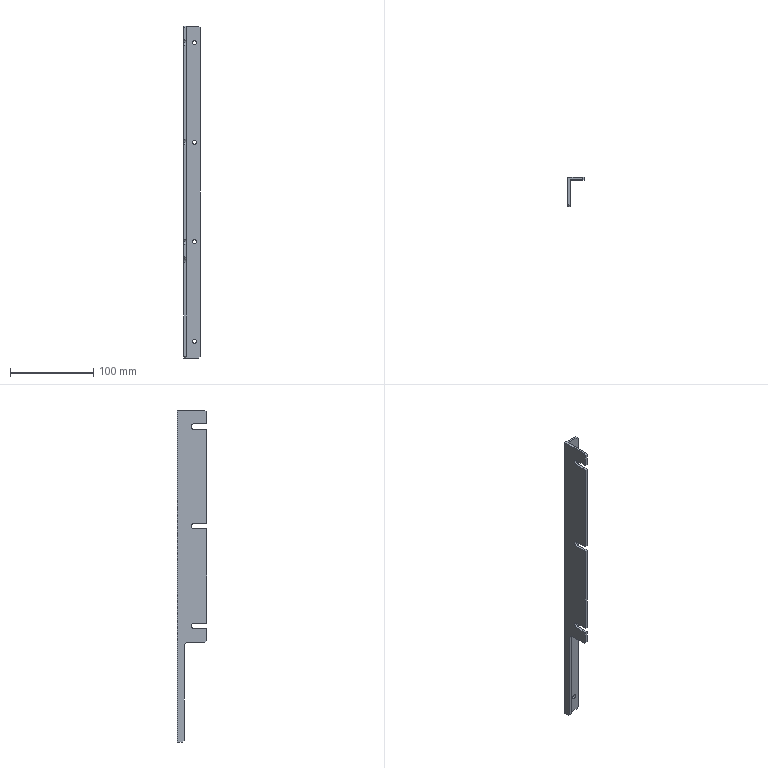Part | SolidWorks | features BaseBody 1 | 1 solid | 39 faces | box 20 x 35 x 400 mm | volume 51386 mm3 | plane 24 | cylinder 15 | commonest cylinder face diameters 5 x8 6.6 x6 10 x1
STEP:
#1=CARTESIAN_POINT('',(13.,32.,377.5));
#2=VERTEX_POINT('',#1);
#3=CARTESIAN_POINT('',(13.,32.,382.5));
#4=VERTEX_POINT('',#3);
#5=CARTESIAN_POINT('',(13.,32.,380.));
#6=DIRECTION('',(0.,1.,0.));
#7=DIRECTION('',(0.,0.,1.));
#8=AXIS2_PLACEMENT_3D('',#5,#6,#7);
#9=CIRCLE('',#8,2.5);
#10=EDGE_CURVE('',#2,#4,#9,.T.);
#11=ORIENTED_EDGE('',*,*,#10,.F.);
#12=CARTESIAN_POINT('',(13.,35.,377.5));
#13=VERTEX_POINT('',#12);
#14=CARTESIAN_POINT('',(13.,35.,377.5));
#15=DIRECTION('',(0.,1.,0.));
#16=VECTOR('',#15,1000.);
#17=LINE('',#14,#16);
#18=EDGE_CURVE('',#2,#13,#17,.T.);
#19=ORIENTED_EDGE('',*,*,#18,.T.);
#20=CARTESIAN_POINT('',(13.,35.,382.5));
#21=VERTEX_POINT('',#20);
#22=CARTESIAN_POINT('',(13.,35.,380.));
#23=DIRECTION('',(0.,1.,0.));
#24=DIRECTION('',(0.,0.,1.));
#25=AXIS2_PLACEMENT_3D('',#22,#23,#24);
#26=CIRCLE('',#25,2.5);
#27=EDGE_CURVE('',#13,#21,#26,.T.);
#28=ORIENTED_EDGE('',*,*,#27,.T.);
#29=CARTESIAN_POINT('',(13.,35.,382.5));
#30=DIRECTION('',(0.,1.,0.));
#31=VECTOR('',#30,1000.);
#32=LINE('',#29,#31);
#33=EDGE_CURVE('',#4,#21,#32,.T.);
#34=ORIENTED_EDGE('',*,*,#33,.F.);
#35=EDGE_LOOP('',(#11,#19,#28,#34));
#36=FACE_OUTER_BOUND('',#35,.T.);
#37=CARTESIAN_POINT('',(13.,35.,380.));
#38=DIRECTION('',(0.,1.,0.));
#39=DIRECTION('',(0.,0.,1.));
#40=AXIS2_PLACEMENT_3D('',#37,#38,#39);
#41=CYLINDRICAL_SURFACE('',#40,2.5);
#42=ADVANCED_FACE('',(#36),#41,.F.);
#43=CARTESIAN_POINT('',(13.,32.,257.5));
#44=VERTEX_POINT('',#43);
#45=CARTESIAN_POINT('',(13.,32.,262.5));
#46=VERTEX_POINT('',#45);
#47=CARTESIAN_POINT('',(13.,32.,260.));
#48=DIRECTION('',(0.,1.,0.));
#49=DIRECTION('',(0.,0.,1.));
#50=AXIS2_PLACEMENT_3D('',#47,#48,#49);
#51=CIRCLE('',#50,2.5);
#52=EDGE_CURVE('',#44,#46,#51,.T.);
#53=ORIENTED_EDGE('',*,*,#52,.F.);
#54=CARTESIAN_POINT('',(13.,35.,257.5));
#55=VERTEX_POINT('',#54);
#56=CARTESIAN_POINT('',(13.,35.,257.5));
#57=DIRECTION('',(0.,1.,0.));
#58=VECTOR('',#57,1000.);
#59=LINE('',#56,#58);
#60=EDGE_CURVE('',#44,#55,#59,.T.);
#61=ORIENTED_EDGE('',*,*,#60,.T.);
#62=CARTESIAN_POINT('',(13.,35.,262.5));
#63=VERTEX_POINT('',#62);
#64=CARTESIAN_POINT('',(13.,35.,260.));
#65=DIRECTION('',(0.,1.,0.));
#66=DIRECTION('',(0.,0.,1.));
#67=AXIS2_PLACEMENT_3D('',#64,#65,#66);
#68=CIRCLE('',#67,2.5);
#69=EDGE_CURVE('',#55,#63,#68,.T.);
#70=ORIENTED_EDGE('',*,*,#69,.T.);
#71=CARTESIAN_POINT('',(13.,35.,262.5));
#72=DIRECTION('',(0.,1.,0.));
#73=VECTOR('',#72,1000.);
#74=LINE('',#71,#73);
#75=EDGE_CURVE('',#46,#63,#74,.T.);
#76=ORIENTED_EDGE('',*,*,#75,.F.);
#77=EDGE_LOOP('',(#53,#61,#70,#76));
#78=FACE_OUTER_BOUND('',#77,.T.);
#79=CARTESIAN_POINT('',(13.,35.,260.));
#80=DIRECTION('',(0.,1.,0.));
#81=DIRECTION('',(0.,0.,1.));
#82=AXIS2_PLACEMENT_3D('',#79,#80,#81);
#83=CYLINDRICAL_SURFACE('',#82,2.5);
#84=ADVANCED_FACE('',(#78),#83,.F.);
#85=CARTESIAN_POINT('',(13.,32.,137.5));
#86=VERTEX_POINT('',#85);
#87=CARTESIAN_POINT('',(13.,32.,142.5));
#88=VERTEX_POINT('',#87);
#89=CARTESIAN_POINT('',(13.,32.,140.));
#90=DIRECTION('',(0.,1.,0.));
#91=DIRECTION('',(0.,0.,1.));
#92=AXIS2_PLACEMENT_3D('',#89,#90,#91);
#93=CIRCLE('',#92,2.5);
#94=EDGE_CURVE('',#86,#88,#93,.T.);
#95=ORIENTED_EDGE('',*,*,#94,.F.);
#96=CARTESIAN_POINT('',(13.,35.,137.5));
#97=VERTEX_POINT('',#96);
#98=CARTESIAN_POINT('',(13.,35.,137.5));
#99=DIRECTION('',(0.,1.,0.));
#100=VECTOR('',#99,1000.);
#101=LINE('',#98,#100);
#102=EDGE_CURVE('',#86,#97,#101,.T.);
#103=ORIENTED_EDGE('',*,*,#102,.T.);
#104=CARTESIAN_POINT('',(13.,35.,142.5));
#105=VERTEX_POINT('',#104);
#106=CARTESIAN_POINT('',(13.,35.,140.));
#107=DIRECTION('',(0.,1.,0.));
#108=DIRECTION('',(0.,0.,1.));
#109=AXIS2_PLACEMENT_3D('',#106,#107,#108);
#110=CIRCLE('',#109,2.5);
#111=EDGE_CURVE('',#97,#105,#110,.T.);
#112=ORIENTED_EDGE('',*,*,#111,.T.);
#113=CARTESIAN_POINT('',(13.,35.,142.5));
#114=DIRECTION('',(0.,1.,0.));
#115=VECTOR('',#114,1000.);
#116=LINE('',#113,#115);
#117=EDGE_CURVE('',#88,#105,#116,.T.);
#118=ORIENTED_EDGE('',*,*,#117,.F.);
#119=EDGE_LOOP('',(#95,#103,#112,#118));
#120=FACE_OUTER_BOUND('',#119,.T.);
#121=CARTESIAN_POINT('',(13.,35.,140.));
#122=DIRECTION('',(0.,1.,0.));
#123=DIRECTION('',(0.,0.,1.));
#124=AXIS2_PLACEMENT_3D('',#121,#122,#123);
#125=CYLINDRICAL_SURFACE('',#124,2.5);
#126=ADVANCED_FACE('',(#120),#125,.F.);
#127=CARTESIAN_POINT('',(13.,32.,17.5));
#128=VERTEX_POINT('',#127);
#129=CARTESIAN_POINT('',(13.,32.,22.5));
#130=VERTEX_POINT('',#129);
#131=CARTESIAN_POINT('',(13.,32.,20.));
#132=DIRECTION('',(0.,1.,0.));
#133=DIRECTION('',(0.,0.,1.));
#134=AXIS2_PLACEMENT_3D('',#131,#132,#133);
#135=CIRCLE('',#134,2.5);
#136=EDGE_CURVE('',#128,#130,#135,.T.);
#137=ORIENTED_EDGE('',*,*,#136,.F.);
#138=CARTESIAN_POINT('',(13.,35.,17.5));
#139=VERTEX_POINT('',#138);
#140=CARTESIAN_POINT('',(13.,35.,17.5));
#141=DIRECTION('',(0.,1.,0.));
#142=VECTOR('',#141,1000.);
#143=LINE('',#140,#142);
#144=EDGE_CURVE('',#128,#139,#143,.T.);
#145=ORIENTED_EDGE('',*,*,#144,.T.);
#146=CARTESIAN_POINT('',(13.,35.,22.5));
#147=VERTEX_POINT('',#146);
#148=CARTESIAN_POINT('',(13.,35.,20.));
#149=DIRECTION('',(0.,1.,0.));
#150=DIRECTION('',(0.,0.,1.));
#151=AXIS2_PLACEMENT_3D('',#148,#149,#150);
#152=CIRCLE('',#151,2.5);
#153=EDGE_CURVE('',#139,#147,#152,.T.);
#154=ORIENTED_EDGE('',*,*,#153,.T.);
#155=CARTESIAN_POINT('',(13.,35.,22.5));
#156=DIRECTION('',(0.,1.,0.));
#157=VECTOR('',#156,1000.);
#158=LINE('',#155,#157);
#159=EDGE_CURVE('',#130,#147,#158,.T.);
#160=ORIENTED_EDGE('',*,*,#159,.F.);
#161=EDGE_LOOP('',(#137,#145,#154,#160));
#162=FACE_OUTER_BOUND('',#161,.T.);
#163=CARTESIAN_POINT('',(13.,35.,20.));
#164=DIRECTION('',(0.,1.,0.));
#165=DIRECTION('',(0.,0.,1.));
#166=AXIS2_PLACEMENT_3D('',#163,#164,#165);
#167=CYLINDRICAL_SURFACE('',#166,2.5);
#168=ADVANCED_FACE('',(#162),#167,.F.);
#169=CARTESIAN_POINT('',(0.,18.3,140.));
#170=VERTEX_POINT('',#169);
#171=CARTESIAN_POINT('',(0.,15.,143.3));
#172=VERTEX_POINT('',#171);
#173=CARTESIAN_POINT('',(0.,15.,140.));
#174=DIRECTION('',(1.,0.,0.));
#175=DIRECTION('',(0.,1.,0.));
#176=AXIS2_PLACEMENT_3D('',#173,#174,#175);
#177=CIRCLE('',#176,3.3);
#178=EDGE_CURVE('',#170,#172,#177,.T.);
#179=ORIENTED_EDGE('',*,*,#178,.F.);
#180=CARTESIAN_POINT('',(3.,18.3,140.));
#181=VERTEX_POINT('',#180);
#182=CARTESIAN_POINT('',(0.,18.3,140.));
#183=DIRECTION('',(1.,0.,0.));
#184=VECTOR('',#183,1000.);
#185=LINE('',#182,#184);
#186=EDGE_CURVE('',#170,#181,#185,.T.);
#187=ORIENTED_EDGE('',*,*,#186,.T.);
#188=CARTESIAN_POINT('',(3.,15.,143.3));
#189=VERTEX_POINT('',#188);
#190=CARTESIAN_POINT('',(3.,15.,140.));
#191=DIRECTION('',(1.,0.,0.));
#192=DIRECTION('',(0.,1.,0.));
#193=AXIS2_PLACEMENT_3D('',#190,#191,#192);
#194=CIRCLE('',#193,3.3);
#195=EDGE_CURVE('',#181,#189,#194,.T.);
#196=ORIENTED_EDGE('',*,*,#195,.T.);
#197=CARTESIAN_POINT('',(0.,15.,143.3));
#198=DIRECTION('',(1.,0.,0.));
#199=VECTOR('',#198,1000.);
#200=LINE('',#197,#199);
#201=EDGE_CURVE('',#172,#189,#200,.T.);
#202=ORIENTED_EDGE('',*,*,#201,.F.);
#203=EDGE_LOOP('',(#179,#187,#196,#202));
#204=FACE_OUTER_BOUND('',#203,.T.);
#205=CARTESIAN_POINT('',(0.,15.,140.));
#206=DIRECTION('',(1.,0.,0.));
#207=DIRECTION('',(0.,1.,0.));
#208=AXIS2_PLACEMENT_3D('',#205,#206,#207);
#209=CYLINDRICAL_SURFACE('',#208,3.3);
#210=ADVANCED_FACE('',(#204),#209,.F.);
#211=CARTESIAN_POINT('',(0.,18.3,380.));
#212=VERTEX_POINT('',#211);
#213=CARTESIAN_POINT('',(0.,15.,383.3));
#214=VERTEX_POINT('',#213);
#215=CARTESIAN_POINT('',(0.,15.,380.));
#216=DIRECTION('',(1.,0.,0.));
#217=DIRECTION('',(0.,1.,0.));
#218=AXIS2_PLACEMENT_3D('',#215,#216,#217);
#219=CIRCLE('',#218,3.3);
#220=EDGE_CURVE('',#212,#214,#219,.T.);
#221=ORIENTED_EDGE('',*,*,#220,.F.);
#222=CARTESIAN_POINT('',(3.,18.3,380.));
#223=VERTEX_POINT('',#222);
#224=CARTESIAN_POINT('',(0.,18.3,380.));
#225=DIRECTION('',(1.,0.,0.));
#226=VECTOR('',#225,1000.);
#227=LINE('',#224,#226);
#228=EDGE_CURVE('',#212,#223,#227,.T.);
#229=ORIENTED_EDGE('',*,*,#228,.T.);
#230=CARTESIAN_POINT('',(3.,15.,383.3));
#231=VERTEX_POINT('',#230);
#232=CARTESIAN_POINT('',(3.,15.,380.));
#233=DIRECTION('',(1.,0.,0.));
#234=DIRECTION('',(0.,1.,0.));
#235=AXIS2_PLACEMENT_3D('',#232,#233,#234);
#236=CIRCLE('',#235,3.3);
#237=EDGE_CURVE('',#223,#231,#236,.T.);
#238=ORIENTED_EDGE('',*,*,#237,.T.);
#239=CARTESIAN_POINT('',(0.,15.,383.3));
#240=DIRECTION('',(1.,0.,0.));
#241=VECTOR('',#240,1000.);
#242=LINE('',#239,#241);
#243=EDGE_CURVE('',#214,#231,#242,.T.);
#244=ORIENTED_EDGE('',*,*,#243,.F.);
#245=EDGE_LOOP('',(#221,#229,#238,#244));
#246=FACE_OUTER_BOUND('',#245,.T.);
#247=CARTESIAN_POINT('',(0.,15.,380.));
#248=DIRECTION('',(1.,0.,0.));
#249=DIRECTION('',(0.,1.,0.));
#250=AXIS2_PLACEMENT_3D('',#247,#248,#249);
#251=CYLINDRICAL_SURFACE('',#250,3.3);
#252=ADVANCED_FACE('',(#246),#251,.F.);
#253=CARTESIAN_POINT('',(0.,18.3,260.));
#254=VERTEX_POINT('',#253);
#255=CARTESIAN_POINT('',(0.,15.,263.3));
#256=VERTEX_POINT('',#255);
#257=CARTESIAN_POINT('',(0.,15.,260.));
#258=DIRECTION('',(1.,0.,0.));
#259=DIRECTION('',(0.,1.,0.));
#260=AXIS2_PLACEMENT_3D('',#257,#258,#259);
#261=CIRCLE('',#260,3.3);
#262=EDGE_CURVE('',#254,#256,#261,.T.);
#263=ORIENTED_EDGE('',*,*,#262,.F.);
#264=CARTESIAN_POINT('',(3.,18.3,260.));
#265=VERTEX_POINT('',#264);
#266=CARTESIAN_POINT('',(0.,18.3,260.));
#267=DIRECTION('',(1.,0.,0.));
#268=VECTOR('',#267,1000.);
#269=LINE('',#266,#268);
#270=EDGE_CURVE('',#254,#265,#269,.T.);
#271=ORIENTED_EDGE('',*,*,#270,.T.);
#272=CARTESIAN_POINT('',(3.,15.,263.3));
#273=VERTEX_POINT('',#272);
#274=CARTESIAN_POINT('',(3.,15.,260.));
#275=DIRECTION('',(1.,0.,0.));
#276=DIRECTION('',(0.,1.,0.));
#277=AXIS2_PLACEMENT_3D('',#274,#275,#276);
#278=CIRCLE('',#277,3.3);
#279=EDGE_CURVE('',#265,#273,#278,.T.);
#280=ORIENTED_EDGE('',*,*,#279,.T.);
#281=CARTESIAN_POINT('',(0.,15.,263.3));
#282=DIRECTION('',(1.,0.,0.));
#283=VECTOR('',#282,1000.);
#284=LINE('',#281,#283);
#285=EDGE_CURVE('',#256,#273,#284,.T.);
#286=ORIENTED_EDGE('',*,*,#285,.F.);
#287=EDGE_LOOP('',(#263,#271,#280,#286));
#288=FACE_OUTER_BOUND('',#287,.T.);
#289=CARTESIAN_POINT('',(0.,15.,260.));
#290=DIRECTION('',(1.,0.,0.));
#291=DIRECTION('',(0.,1.,0.));
#292=AXIS2_PLACEMENT_3D('',#289,#290,#291);
#293=CYLINDRICAL_SURFACE('',#292,3.3);
#294=ADVANCED_FACE('',(#288),#293,.F.);
#295=CARTESIAN_POINT('',(0.,27.,115.));
#296=VERTEX_POINT('',#295);
#297=CARTESIAN_POINT('',(0.,22.,120.));
#298=VERTEX_POINT('',#297);
#299=CARTESIAN_POINT('',(0.,22.,115.));
#300=DIRECTION('',(1.,0.,0.));
#301=DIRECTION('',(0.,0.,-1.));
#302=AXIS2_PLACEMENT_3D('',#299,#300,#301);
#303=CIRCLE('',#302,5.);
#304=EDGE_CURVE('',#296,#298,#303,.T.);
#305=ORIENTED_EDGE('',*,*,#304,.F.);
#306=CARTESIAN_POINT('',(3.,27.,115.));
#307=VERTEX_POINT('',#306);
#308=CARTESIAN_POINT('',(0.,27.,115.));
#309=DIRECTION('',(-1.,0.,0.));
#310=VECTOR('',#309,1000.);
#311=LINE('',#308,#310);
#312=EDGE_CURVE('',#307,#296,#311,.T.);
#313=ORIENTED_EDGE('',*,*,#312,.F.);
#314=CARTESIAN_POINT('',(3.,22.,120.));
#315=VERTEX_POINT('',#314);
#316=CARTESIAN_POINT('',(3.,22.,115.));
#317=DIRECTION('',(-1.,0.,0.));
#318=DIRECTION('',(0.,-1.,0.));
#319=AXIS2_PLACEMENT_3D('',#316,#317,#318);
#320=CIRCLE('',#319,5.);
#321=EDGE_CURVE('',#315,#307,#320,.T.);
#322=ORIENTED_EDGE('',*,*,#321,.F.);
#323=CARTESIAN_POINT('',(3.,22.,120.));
#324=DIRECTION('',(1.,0.,0.));
#325=VECTOR('',#324,1000.);
#326=LINE('',#323,#325);
#327=EDGE_CURVE('',#298,#315,#326,.T.);
#328=ORIENTED_EDGE('',*,*,#327,.F.);
#329=EDGE_LOOP('',(#305,#313,#322,#328));
#330=FACE_OUTER_BOUND('',#329,.T.);
#331=CARTESIAN_POINT('',(0.,22.,115.));
#332=DIRECTION('',(-1.,0.,0.));
#333=DIRECTION('',(0.,-1.,0.));
#334=AXIS2_PLACEMENT_3D('',#331,#332,#333);
#335=CYLINDRICAL_SURFACE('',#334,5.);
#336=ADVANCED_FACE('',(#330),#335,.F.);
#337=CARTESIAN_POINT('',(18.,32.,0.));
#338=VERTEX_POINT('',#337);
#339=CARTESIAN_POINT('',(20.,32.,2.));
#340=VERTEX_POINT('',#339);
#341=CARTESIAN_POINT('',(20.,32.,2.));
#342=DIRECTION('',(0.7071,0.,0.7071));
#343=VECTOR('',#342,1000.);
#344=LINE('',#341,#343);
#345=EDGE_CURVE('',#338,#340,#344,.T.);
#346=ORIENTED_EDGE('',*,*,#345,.F.);
#347=CARTESIAN_POINT('',(18.,35.,0.));
#348=VERTEX_POINT('',#347);
#349=CARTESIAN_POINT('',(18.,32.,0.));
#350=DIRECTION('',(0.,-1.,0.));
#351=VECTOR('',#350,1000.);
#352=LINE('',#349,#351);
#353=EDGE_CURVE('',#348,#338,#352,.T.);
#354=ORIENTED_EDGE('',*,*,#353,.F.);
#355=CARTESIAN_POINT('',(20.,35.,2.));
#356=VERTEX_POINT('',#355);
#357=CARTESIAN_POINT('',(20.,35.,2.));
#358=DIRECTION('',(-0.7071,0.,-0.7071));
#359=VECTOR('',#358,1000.);
#360=LINE('',#357,#359);
#361=EDGE_CURVE('',#356,#348,#360,.T.);
#362=ORIENTED_EDGE('',*,*,#361,.F.);
#363=CARTESIAN_POINT('',(20.,35.,2.));
#364=DIRECTION('',(0.,1.,0.));
#365=VECTOR('',#364,1000.);
#366=LINE('',#363,#365);
#367=EDGE_CURVE('',#340,#356,#366,.T.);
#368=ORIENTED_EDGE('',*,*,#367,.F.);
#369=EDGE_LOOP('',(#346,#354,#362,#368));
#370=FACE_OUTER_BOUND('',#369,.T.);
#371=CARTESIAN_POINT('',(20.,35.,2.));
#372=DIRECTION('',(0.7071,0.,-0.7071));
#373=DIRECTION('',(0.,-1.,0.));
#374=AXIS2_PLACEMENT_3D('',#371,#372,#373);
#375=PLANE('',#374);
#376=ADVANCED_FACE('',(#370),#375,.T.);
#377=CARTESIAN_POINT('',(0.,29.,0.));
#378=VERTEX_POINT('',#377);
#379=CARTESIAN_POINT('',(0.,27.,2.));
#380=VERTEX_POINT('',#379);
#381=CARTESIAN_POINT('',(0.,27.,2.));
#382=DIRECTION('',(0.,-0.7071,0.7071));
#383=VECTOR('',#382,1000.);
#384=LINE('',#381,#383);
#385=EDGE_CURVE('',#378,#380,#384,.T.);
#386=ORIENTED_EDGE('',*,*,#385,.F.);
#387=CARTESIAN_POINT('',(3.,29.,0.));
#388=VERTEX_POINT('',#387);
#389=CARTESIAN_POINT('',(0.,29.,0.));
#390=DIRECTION('',(-1.,0.,0.));
#391=VECTOR('',#390,1000.);
#392=LINE('',#389,#391);
#393=EDGE_CURVE('',#388,#378,#392,.T.);
#394=ORIENTED_EDGE('',*,*,#393,.F.);
#395=CARTESIAN_POINT('',(3.,27.,2.));
#396=VERTEX_POINT('',#395);
#397=CARTESIAN_POINT('',(3.,27.,2.));
#398=DIRECTION('',(0.,0.7071,-0.7071));
#399=VECTOR('',#398,1000.);
#400=LINE('',#397,#399);
#401=EDGE_CURVE('',#396,#388,#400,.T.);
#402=ORIENTED_EDGE('',*,*,#401,.F.);
#403=CARTESIAN_POINT('',(3.,27.,2.));
#404=DIRECTION('',(1.,0.,0.));
#405=VECTOR('',#404,1000.);
#406=LINE('',#403,#405);
#407=EDGE_CURVE('',#380,#396,#406,.T.);
#408=ORIENTED_EDGE('',*,*,#407,.F.);
#409=EDGE_LOOP('',(#386,#394,#402,#408));
#410=FACE_OUTER_BOUND('',#409,.T.);
#411=CARTESIAN_POINT('',(0.,27.,2.));
#412=DIRECTION('',(0.,-0.7071,-0.7071));
#413=DIRECTION('',(0.,-0.7071,0.7071));
#414=AXIS2_PLACEMENT_3D('',#411,#412,#413);
#415=PLANE('',#414);
#416=ADVANCED_FACE('',(#410),#415,.T.);
#417=CARTESIAN_POINT('',(0.,2.,120.));
#418=VERTEX_POINT('',#417);
#419=CARTESIAN_POINT('',(0.,0.,122.));
#420=VERTEX_POINT('',#419);
#421=CARTESIAN_POINT('',(0.,0.,122.));
#422=DIRECTION('',(0.,-0.7071,0.7071));
#423=VECTOR('',#422,1000.);
#424=LINE('',#421,#423);
#425=EDGE_CURVE('',#418,#420,#424,.T.);
#426=ORIENTED_EDGE('',*,*,#425,.F.);
#427=CARTESIAN_POINT('',(3.,2.,120.));
#428=VERTEX_POINT('',#427);
#429=CARTESIAN_POINT('',(0.,2.,120.));
#430=DIRECTION('',(-1.,0.,0.));
#431=VECTOR('',#430,1000.);
#432=LINE('',#429,#431);
#433=EDGE_CURVE('',#428,#418,#432,.T.);
#434=ORIENTED_EDGE('',*,*,#433,.F.);
#435=CARTESIAN_POINT('',(3.,0.,122.));
#436=VERTEX_POINT('',#435);
#437=CARTESIAN_POINT('',(3.,0.,122.));
#438=DIRECTION('',(0.,0.7071,-0.7071));
#439=VECTOR('',#438,1000.);
#440=LINE('',#437,#439);
#441=EDGE_CURVE('',#436,#428,#440,.T.);
#442=ORIENTED_EDGE('',*,*,#441,.F.);
#443=CARTESIAN_POINT('',(3.,0.,122.));
#444=DIRECTION('',(1.,0.,0.));
#445=VECTOR('',#444,1000.);
#446=LINE('',#443,#445);
#447=EDGE_CURVE('',#420,#436,#446,.T.);
#448=ORIENTED_EDGE('',*,*,#447,.F.);
#449=EDGE_LOOP('',(#426,#434,#442,#448));
#450=FACE_OUTER_BOUND('',#449,.T.);
#451=CARTESIAN_POINT('',(3.,0.,122.));
#452=DIRECTION('',(0.,0.7071,0.7071));
#453=DIRECTION('',(1.,0.,0.));
#454=AXIS2_PLACEMENT_3D('',#451,#452,#453);
#455=PLANE('',#454);
#456=ADVANCED_FACE('',(#450),#455,.F.);
#457=CARTESIAN_POINT('',(0.,0.,398.));
#458=VERTEX_POINT('',#457);
#459=CARTESIAN_POINT('',(0.,2.,400.));
#460=VERTEX_POINT('',#459);
#461=CARTESIAN_POINT('',(0.,2.,400.));
#462=DIRECTION('',(0.,0.7071,0.7071));
#463=VECTOR('',#462,1000.);
#464=LINE('',#461,#463);
#465=EDGE_CURVE('',#458,#460,#464,.T.);
#466=ORIENTED_EDGE('',*,*,#465,.F.);
#467=CARTESIAN_POINT('',(3.,0.,398.));
#468=VERTEX_POINT('',#467);
#469=CARTESIAN_POINT('',(3.,0.,398.));
#470=DIRECTION('',(-1.,0.,0.));
#471=VECTOR('',#470,1000.);
#472=LINE('',#469,#471);
#473=EDGE_CURVE('',#468,#458,#472,.T.);
#474=ORIENTED_EDGE('',*,*,#473,.F.);
#475=CARTESIAN_POINT('',(3.,2.,400.));
#476=VERTEX_POINT('',#475);
#477=CARTESIAN_POINT('',(3.,2.,400.));
#478=DIRECTION('',(0.,-0.7071,-0.7071));
#479=VECTOR('',#478,1000.);
#480=LINE('',#477,#479);
#481=EDGE_CURVE('',#476,#468,#480,.T.);
#482=ORIENTED_EDGE('',*,*,#481,.F.);
#483=CARTESIAN_POINT('',(0.,2.,400.));
#484=DIRECTION('',(1.,0.,0.));
#485=VECTOR('',#484,1000.);
#486=LINE('',#483,#485);
#487=EDGE_CURVE('',#460,#476,#486,.T.);
#488=ORIENTED_EDGE('',*,*,#487,.F.);
#489=EDGE_LOOP('',(#466,#474,#482,#488));
#490=FACE_OUTER_BOUND('',#489,.T.);
#491=CARTESIAN_POINT('',(0.,2.,400.));
#492=DIRECTION('',(0.,0.7071,-0.7071));
#493=DIRECTION('',(-1.,0.,0.));
#494=AXIS2_PLACEMENT_3D('',#491,#492,#493);
#495=PLANE('',#494);
#496=ADVANCED_FACE('',(#490),#495,.F.);
#497=CARTESIAN_POINT('',(20.,32.,398.));
#498=VERTEX_POINT('',#497);
#499=CARTESIAN_POINT('',(18.,32.,400.));
#500=VERTEX_POINT('',#499);
#501=CARTESIAN_POINT('',(18.,32.,400.));
#502=DIRECTION('',(-0.7071,0.,0.7071));
#503=VECTOR('',#502,1000.);
#504=LINE('',#501,#503);
#505=EDGE_CURVE('',#498,#500,#504,.T.);
#506=ORIENTED_EDGE('',*,*,#505,.F.);
#507=CARTESIAN_POINT('',(20.,35.,398.));
#508=VERTEX_POINT('',#507);
#509=CARTESIAN_POINT('',(20.,35.,398.));
#510=DIRECTION('',(0.,-1.,0.));
#511=VECTOR('',#510,1000.);
#512=LINE('',#509,#511);
#513=EDGE_CURVE('',#508,#498,#512,.T.);
#514=ORIENTED_EDGE('',*,*,#513,.F.);
#515=CARTESIAN_POINT('',(18.,35.,400.));
#516=VERTEX_POINT('',#515);
#517=CARTESIAN_POINT('',(18.,35.,400.));
#518=DIRECTION('',(0.7071,0.,-0.7071));
#519=VECTOR('',#518,1000.);
#520=LINE('',#517,#519);
#521=EDGE_CURVE('',#516,#508,#520,.T.);
#522=ORIENTED_EDGE('',*,*,#521,.F.);
#523=CARTESIAN_POINT('',(18.,0.,400.));
#524=DIRECTION('',(0.,1.,0.));
#525=VECTOR('',#524,1000.);
#526=LINE('',#523,#525);
#527=EDGE_CURVE('',#500,#516,#526,.T.);
#528=ORIENTED_EDGE('',*,*,#527,.F.);
#529=EDGE_LOOP('',(#506,#514,#522,#528));
#530=FACE_OUTER_BOUND('',#529,.T.);
#531=CARTESIAN_POINT('',(18.,0.,400.));
#532=DIRECTION('',(-0.7071,0.,-0.7071));
#533=DIRECTION('',(-0.7071,0.,0.7071));
#534=AXIS2_PLACEMENT_3D('',#531,#532,#533);
#535=PLANE('',#534);
#536=ADVANCED_FACE('',(#530),#535,.F.);
#537=CARTESIAN_POINT('',(3.,27.,0.));
#538=DIRECTION('',(0.,0.,1.));
#539=VECTOR('',#538,1000.);
#540=LINE('',#537,#539);
#541=EDGE_CURVE('',#396,#307,#540,.T.);
#542=ORIENTED_EDGE('',*,*,#541,.T.);
#543=ORIENTED_EDGE('',*,*,#312,.T.);
#544=CARTESIAN_POINT('',(0.,27.,0.));
#545=DIRECTION('',(0.,0.,1.));
#546=VECTOR('',#545,1000.);
#547=LINE('',#544,#546);
#548=EDGE_CURVE('',#380,#296,#547,.T.);
#549=ORIENTED_EDGE('',*,*,#548,.F.);
#550=ORIENTED_EDGE('',*,*,#407,.T.);
#551=EDGE_LOOP('',(#542,#543,#549,#550));
#552=FACE_OUTER_BOUND('',#551,.T.);
#553=CARTESIAN_POINT('',(0.,27.,0.));
#554=DIRECTION('',(0.,1.,0.));
#555=DIRECTION('',(1.,0.,0.));
#556=AXIS2_PLACEMENT_3D('',#553,#554,#555);
#557=PLANE('',#556);
#558=ADVANCED_FACE('',(#552),#557,.F.);
#559=CARTESIAN_POINT('',(0.,0.,120.));
#560=DIRECTION('',(0.,-1.,0.));
#561=VECTOR('',#560,1000.);
#562=LINE('',#559,#561);
#563=EDGE_CURVE('',#298,#418,#562,.T.);
#564=ORIENTED_EDGE('',*,*,#563,.F.);
#565=ORIENTED_EDGE('',*,*,#327,.T.);
#566=CARTESIAN_POINT('',(3.,0.,120.));
#567=DIRECTION('',(0.,-1.,0.));
#568=VECTOR('',#567,1000.);
#569=LINE('',#566,#568);
#570=EDGE_CURVE('',#315,#428,#569,.T.);
#571=ORIENTED_EDGE('',*,*,#570,.T.);
#572=ORIENTED_EDGE('',*,*,#433,.T.);
#573=EDGE_LOOP('',(#564,#565,#571,#572));
#574=FACE_OUTER_BOUND('',#573,.T.);
#575=CARTESIAN_POINT('',(0.,0.,120.));
#576=DIRECTION('',(0.,0.,1.));
#577=DIRECTION('',(1.,0.,0.));
#578=AXIS2_PLACEMENT_3D('',#575,#576,#577);
#579=PLANE('',#578);
#580=ADVANCED_FACE('',(#574),#579,.F.);
#581=CARTESIAN_POINT('',(3.,0.,136.7));
#582=VERTEX_POINT('',#581);
#583=CARTESIAN_POINT('',(3.,15.,136.7));
#584=VERTEX_POINT('',#583);
#585=CARTESIAN_POINT('',(3.,0.,136.7));
#586=DIRECTION('',(0.,1.,0.));
#587=VECTOR('',#586,1000.);
#588=LINE('',#585,#587);
#589=EDGE_CURVE('',#582,#584,#588,.T.);
#590=ORIENTED_EDGE('',*,*,#589,.T.);
#591=CARTESIAN_POINT('',(0.,15.,136.7));
#592=VERTEX_POINT('',#591);
#593=CARTESIAN_POINT('',(0.,15.,136.7));
#594=DIRECTION('',(1.,0.,0.));
#595=VECTOR('',#594,1000.);
#596=LINE('',#593,#595);
#597=EDGE_CURVE('',#592,#584,#596,.T.);
#598=ORIENTED_EDGE('',*,*,#597,.F.);
#599=CARTESIAN_POINT('',(0.,0.,136.7));
#600=VERTEX_POINT('',#599);
#601=CARTESIAN_POINT('',(0.,0.,136.7));
#602=DIRECTION('',(0.,1.,0.));
#603=VECTOR('',#602,1000.);
#604=LINE('',#601,#603);
#605=EDGE_CURVE('',#600,#592,#604,.T.);
#606=ORIENTED_EDGE('',*,*,#605,.F.);
#607=CARTESIAN_POINT('',(0.,0.,136.7));
#608=DIRECTION('',(1.,0.,0.));
#609=VECTOR('',#608,1000.);
#610=LINE('',#607,#609);
#611=EDGE_CURVE('',#600,#582,#610,.T.);
#612=ORIENTED_EDGE('',*,*,#611,.T.);
#613=EDGE_LOOP('',(#590,#598,#606,#612));
#614=FACE_OUTER_BOUND('',#613,.T.);
#615=CARTESIAN_POINT('',(0.,0.,136.7));
#616=DIRECTION('',(0.,0.,-1.));
#617=DIRECTION('',(-1.,0.,0.));
#618=AXIS2_PLACEMENT_3D('',#615,#616,#617);
#619=PLANE('',#618);
#620=ADVANCED_FACE('',(#614),#619,.F.);
#621=CARTESIAN_POINT('',(3.,0.,143.3));
#622=VERTEX_POINT('',#621);
#623=CARTESIAN_POINT('',(3.,0.,143.3));
#624=DIRECTION('',(0.,-1.,0.));
#625=VECTOR('',#624,1000.);
#626=LINE('',#623,#625);
#627=EDGE_CURVE('',#189,#622,#626,.T.);
#628=ORIENTED_EDGE('',*,*,#627,.T.);
#629=CARTESIAN_POINT('',(0.,0.,143.3));
#630=VERTEX_POINT('',#629);
#631=CARTESIAN_POINT('',(0.,0.,143.3));
#632=DIRECTION('',(1.,0.,0.));
#633=VECTOR('',#632,1000.);
#634=LINE('',#631,#633);
#635=EDGE_CURVE('',#630,#622,#634,.T.);
#636=ORIENTED_EDGE('',*,*,#635,.F.);
#637=CARTESIAN_POINT('',(0.,0.,143.3));
#638=DIRECTION('',(0.,-1.,0.));
#639=VECTOR('',#638,1000.);
#640=LINE('',#637,#639);
#641=EDGE_CURVE('',#172,#630,#640,.T.);
#642=ORIENTED_EDGE('',*,*,#641,.F.);
#643=ORIENTED_EDGE('',*,*,#201,.T.);
#644=EDGE_LOOP('',(#628,#636,#642,#643));
#645=FACE_OUTER_BOUND('',#644,.T.);
#646=CARTESIAN_POINT('',(0.,0.,143.3));
#647=DIRECTION('',(0.,0.,1.));
#648=DIRECTION('',(0.,-1.,0.));
#649=AXIS2_PLACEMENT_3D('',#646,#647,#648);
#650=PLANE('',#649);
#651=ADVANCED_FACE('',(#645),#650,.F.);
#652=CARTESIAN_POINT('',(3.,0.,376.7));
#653=VERTEX_POINT('',#652);
#654=CARTESIAN_POINT('',(3.,15.,376.7));
#655=VERTEX_POINT('',#654);
#656=CARTESIAN_POINT('',(3.,0.,376.7));
#657=DIRECTION('',(0.,1.,0.));
#658=VECTOR('',#657,1000.);
#659=LINE('',#656,#658);
#660=EDGE_CURVE('',#653,#655,#659,.T.);
#661=ORIENTED_EDGE('',*,*,#660,.T.);
#662=CARTESIAN_POINT('',(0.,15.,376.7));
#663=VERTEX_POINT('',#662);
#664=CARTESIAN_POINT('',(0.,15.,376.7));
#665=DIRECTION('',(1.,0.,0.));
#666=VECTOR('',#665,1000.);
#667=LINE('',#664,#666);
#668=EDGE_CURVE('',#663,#655,#667,.T.);
#669=ORIENTED_EDGE('',*,*,#668,.F.);
#670=CARTESIAN_POINT('',(0.,0.,376.7));
#671=VERTEX_POINT('',#670);
#672=CARTESIAN_POINT('',(0.,0.,376.7));
#673=DIRECTION('',(0.,1.,0.));
#674=VECTOR('',#673,1000.);
#675=LINE('',#672,#674);
#676=EDGE_CURVE('',#671,#663,#675,.T.);
#677=ORIENTED_EDGE('',*,*,#676,.F.);
#678=CARTESIAN_POINT('',(0.,0.,376.7));
#679=DIRECTION('',(1.,0.,0.));
#680=VECTOR('',#679,1000.);
#681=LINE('',#678,#680);
#682=EDGE_CURVE('',#671,#653,#681,.T.);
#683=ORIENTED_EDGE('',*,*,#682,.T.);
#684=EDGE_LOOP('',(#661,#669,#677,#683));
#685=FACE_OUTER_BOUND('',#684,.T.);
#686=CARTESIAN_POINT('',(0.,0.,376.7));
#687=DIRECTION('',(0.,0.,-1.));
#688=DIRECTION('',(0.,-1.,0.));
#689=AXIS2_PLACEMENT_3D('',#686,#687,#688);
#690=PLANE('',#689);
#691=ADVANCED_FACE('',(#685),#690,.F.);
#692=CARTESIAN_POINT('',(3.,0.,383.3));
#693=VERTEX_POINT('',#692);
#694=CARTESIAN_POINT('',(3.,0.,383.3));
#695=DIRECTION('',(0.,-1.,0.));
#696=VECTOR('',#695,1000.);
#697=LINE('',#694,#696);
#698=EDGE_CURVE('',#231,#693,#697,.T.);
#699=ORIENTED_EDGE('',*,*,#698,.T.);
#700=CARTESIAN_POINT('',(0.,0.,383.3));
#701=VERTEX_POINT('',#700);
#702=CARTESIAN_POINT('',(0.,0.,383.3));
#703=DIRECTION('',(1.,0.,0.));
#704=VECTOR('',#703,1000.);
#705=LINE('',#702,#704);
#706=EDGE_CURVE('',#701,#693,#705,.T.);
#707=ORIENTED_EDGE('',*,*,#706,.F.);
#708=CARTESIAN_POINT('',(0.,0.,383.3));
#709=DIRECTION('',(0.,-1.,0.));
#710=VECTOR('',#709,1000.);
#711=LINE('',#708,#710);
#712=EDGE_CURVE('',#214,#701,#711,.T.);
#713=ORIENTED_EDGE('',*,*,#712,.F.);
#714=ORIENTED_EDGE('',*,*,#243,.T.);
#715=EDGE_LOOP('',(#699,#707,#713,#714));
#716=FACE_OUTER_BOUND('',#715,.T.);
#717=CARTESIAN_POINT('',(0.,0.,383.3));
#718=DIRECTION('',(0.,0.,1.));
#719=DIRECTION('',(0.,-1.,0.));
#720=AXIS2_PLACEMENT_3D('',#717,#718,#719);
#721=PLANE('',#720);
#722=ADVANCED_FACE('',(#716),#721,.F.);
#723=CARTESIAN_POINT('',(3.,0.,263.3));
#724=VERTEX_POINT('',#723);
#725=CARTESIAN_POINT('',(3.,15.,263.3));
#726=DIRECTION('',(0.,-1.,0.));
#727=VECTOR('',#726,1000.);
#728=LINE('',#725,#727);
#729=EDGE_CURVE('',#273,#724,#728,.T.);
#730=ORIENTED_EDGE('',*,*,#729,.T.);
#731=CARTESIAN_POINT('',(0.,0.,263.3));
#732=VERTEX_POINT('',#731);
#733=CARTESIAN_POINT('',(0.,0.,263.3));
#734=DIRECTION('',(1.,0.,0.));
#735=VECTOR('',#734,1000.);
#736=LINE('',#733,#735);
#737=EDGE_CURVE('',#732,#724,#736,.T.);
#738=ORIENTED_EDGE('',*,*,#737,.F.);
#739=CARTESIAN_POINT('',(0.,15.,263.3));
#740=DIRECTION('',(0.,-1.,0.));
#741=VECTOR('',#740,1000.);
#742=LINE('',#739,#741);
#743=EDGE_CURVE('',#256,#732,#742,.T.);
#744=ORIENTED_EDGE('',*,*,#743,.F.);
#745=ORIENTED_EDGE('',*,*,#285,.T.);
#746=EDGE_LOOP('',(#730,#738,#744,#745));
#747=FACE_OUTER_BOUND('',#746,.T.);
#748=CARTESIAN_POINT('',(0.,15.,263.3));
#749=DIRECTION('',(0.,0.,1.));
#750=DIRECTION('',(0.,-1.,0.));
#751=AXIS2_PLACEMENT_3D('',#748,#749,#750);
#752=PLANE('',#751);
#753=ADVANCED_FACE('',(#747),#752,.F.);
#754=CARTESIAN_POINT('',(3.,0.,256.7));
#755=VERTEX_POINT('',#754);
#756=CARTESIAN_POINT('',(3.,15.,256.7));
#757=VERTEX_POINT('',#756);
#758=CARTESIAN_POINT('',(3.,15.,256.7));
#759=DIRECTION('',(0.,1.,0.));
#760=VECTOR('',#759,1000.);
#761=LINE('',#758,#760);
#762=EDGE_CURVE('',#755,#757,#761,.T.);
#763=ORIENTED_EDGE('',*,*,#762,.T.);
#764=CARTESIAN_POINT('',(0.,15.,256.7));
#765=VERTEX_POINT('',#764);
#766=CARTESIAN_POINT('',(0.,15.,256.7));
#767=DIRECTION('',(1.,0.,0.));
#768=VECTOR('',#767,1000.);
#769=LINE('',#766,#768);
#770=EDGE_CURVE('',#765,#757,#769,.T.);
#771=ORIENTED_EDGE('',*,*,#770,.F.);
#772=CARTESIAN_POINT('',(0.,0.,256.7));
#773=VERTEX_POINT('',#772);
#774=CARTESIAN_POINT('',(0.,15.,256.7));
#775=DIRECTION('',(0.,1.,0.));
#776=VECTOR('',#775,1000.);
#777=LINE('',#774,#776);
#778=EDGE_CURVE('',#773,#765,#777,.T.);
#779=ORIENTED_EDGE('',*,*,#778,.F.);
#780=CARTESIAN_POINT('',(0.,0.,256.7));
#781=DIRECTION('',(1.,0.,0.));
#782=VECTOR('',#781,1000.);
#783=LINE('',#780,#782);
#784=EDGE_CURVE('',#773,#755,#783,.T.);
#785=ORIENTED_EDGE('',*,*,#784,.T.);
#786=EDGE_LOOP('',(#763,#771,#779,#785));
#787=FACE_OUTER_BOUND('',#786,.T.);
#788=CARTESIAN_POINT('',(0.,15.,256.7));
#789=DIRECTION('',(0.,0.,-1.));
#790=DIRECTION('',(-1.,0.,0.));
#791=AXIS2_PLACEMENT_3D('',#788,#789,#790);
#792=PLANE('',#791);
#793=ADVANCED_FACE('',(#787),#792,.F.);
#794=CARTESIAN_POINT('',(3.,32.,0.));
#795=VERTEX_POINT('',#794);
#796=CARTESIAN_POINT('',(3.,32.,0.));
#797=DIRECTION('',(0.,1.,0.));
#798=VECTOR('',#797,1000.);
#799=LINE('',#796,#798);
#800=EDGE_CURVE('',#388,#795,#799,.T.);
#801=ORIENTED_EDGE('',*,*,#800,.F.);
#802=ORIENTED_EDGE('',*,*,#393,.T.);
#803=CARTESIAN_POINT('',(0.,35.,0.));
#804=VERTEX_POINT('',#803);
#805=CARTESIAN_POINT('',(0.,0.,0.));
#806=DIRECTION('',(0.,-1.,0.));
#807=VECTOR('',#806,1000.);
#808=LINE('',#805,#807);
#809=EDGE_CURVE('',#804,#378,#808,.T.);
#810=ORIENTED_EDGE('',*,*,#809,.F.);
#811=CARTESIAN_POINT('',(0.,35.,0.));
#812=DIRECTION('',(-1.,0.,0.));
#813=VECTOR('',#812,1000.);
#814=LINE('',#811,#813);
#815=EDGE_CURVE('',#348,#804,#814,.T.);
#816=ORIENTED_EDGE('',*,*,#815,.F.);
#817=ORIENTED_EDGE('',*,*,#353,.T.);
#818=CARTESIAN_POINT('',(20.,32.,0.));
#819=DIRECTION('',(1.,0.,0.));
#820=VECTOR('',#819,1000.);
#821=LINE('',#818,#820);
#822=EDGE_CURVE('',#795,#338,#821,.T.);
#823=ORIENTED_EDGE('',*,*,#822,.F.);
#824=EDGE_LOOP('',(#801,#802,#810,#816,#817,#823));
#825=FACE_OUTER_BOUND('',#824,.T.);
#826=CARTESIAN_POINT('',(0.,0.,0.));
#827=DIRECTION('',(0.,0.,-1.));
#828=DIRECTION('',(0.,-1.,0.));
#829=AXIS2_PLACEMENT_3D('',#826,#827,#828);
#830=PLANE('',#829);
#831=ADVANCED_FACE('',(#825),#830,.T.);
#832=CARTESIAN_POINT('',(3.,32.,400.));
#833=VERTEX_POINT('',#832);
#834=CARTESIAN_POINT('',(20.,32.,400.));
#835=DIRECTION('',(1.,0.,0.));
#836=VECTOR('',#835,1000.);
#837=LINE('',#834,#836);
#838=EDGE_CURVE('',#833,#500,#837,.T.);
#839=ORIENTED_EDGE('',*,*,#838,.T.);
#840=ORIENTED_EDGE('',*,*,#527,.T.);
#841=CARTESIAN_POINT('',(0.,35.,400.));
#842=VERTEX_POINT('',#841);
#843=CARTESIAN_POINT('',(0.,35.,400.));
#844=DIRECTION('',(-1.,0.,0.));
#845=VECTOR('',#844,1000.);
#846=LINE('',#843,#845);
#847=EDGE_CURVE('',#516,#842,#846,.T.);
#848=ORIENTED_EDGE('',*,*,#847,.T.);
#849=CARTESIAN_POINT('',(0.,0.,400.));
#850=DIRECTION('',(0.,-1.,0.));
#851=VECTOR('',#850,1000.);
#852=LINE('',#849,#851);
#853=EDGE_CURVE('',#842,#460,#852,.T.);
#854=ORIENTED_EDGE('',*,*,#853,.T.);
#855=ORIENTED_EDGE('',*,*,#487,.T.);
#856=CARTESIAN_POINT('',(3.,32.,400.));
#857=DIRECTION('',(0.,1.,0.));
#858=VECTOR('',#857,1000.);
#859=LINE('',#856,#858);
#860=EDGE_CURVE('',#476,#833,#859,.T.);
#861=ORIENTED_EDGE('',*,*,#860,.T.);
#862=EDGE_LOOP('',(#839,#840,#848,#854,#855,#861));
#863=FACE_OUTER_BOUND('',#862,.T.);
#864=CARTESIAN_POINT('',(0.,0.,400.));
#865=DIRECTION('',(0.,0.,-1.));
#866=DIRECTION('',(0.,-1.,0.));
#867=AXIS2_PLACEMENT_3D('',#864,#865,#866);
#868=PLANE('',#867);
#869=ADVANCED_FACE('',(#863),#868,.F.);
#870=CARTESIAN_POINT('',(0.,0.,400.));
#871=DIRECTION('',(0.,0.,-1.));
#872=VECTOR('',#871,1000.);
#873=LINE('',#870,#872);
#874=EDGE_CURVE('',#458,#701,#873,.T.);
#875=ORIENTED_EDGE('',*,*,#874,.F.);
#876=ORIENTED_EDGE('',*,*,#465,.T.);
#877=ORIENTED_EDGE('',*,*,#853,.F.);
#878=CARTESIAN_POINT('',(0.,35.,400.));
#879=DIRECTION('',(0.,0.,-1.));
#880=VECTOR('',#879,1000.);
#881=LINE('',#878,#880);
#882=EDGE_CURVE('',#842,#804,#881,.T.);
#883=ORIENTED_EDGE('',*,*,#882,.T.);
#884=ORIENTED_EDGE('',*,*,#809,.T.);
#885=ORIENTED_EDGE('',*,*,#385,.T.);
#886=ORIENTED_EDGE('',*,*,#548,.T.);
#887=ORIENTED_EDGE('',*,*,#304,.T.);
#888=ORIENTED_EDGE('',*,*,#563,.T.);
#889=ORIENTED_EDGE('',*,*,#425,.T.);
#890=CARTESIAN_POINT('',(0.,0.,400.));
#891=DIRECTION('',(0.,0.,-1.));
#892=VECTOR('',#891,1000.);
#893=LINE('',#890,#892);
#894=EDGE_CURVE('',#600,#420,#893,.T.);
#895=ORIENTED_EDGE('',*,*,#894,.F.);
#896=ORIENTED_EDGE('',*,*,#605,.T.);
#897=CARTESIAN_POINT('',(0.,15.,140.));
#898=DIRECTION('',(1.,0.,0.));
#899=DIRECTION('',(0.,1.,0.));
#900=AXIS2_PLACEMENT_3D('',#897,#898,#899);
#901=CIRCLE('',#900,3.3);
#902=EDGE_CURVE('',#592,#170,#901,.T.);
#903=ORIENTED_EDGE('',*,*,#902,.T.);
#904=ORIENTED_EDGE('',*,*,#178,.T.);
#905=ORIENTED_EDGE('',*,*,#641,.T.);
#906=CARTESIAN_POINT('',(0.,0.,400.));
#907=DIRECTION('',(0.,0.,-1.));
#908=VECTOR('',#907,1000.);
#909=LINE('',#906,#908);
#910=EDGE_CURVE('',#773,#630,#909,.T.);
#911=ORIENTED_EDGE('',*,*,#910,.F.);
#912=ORIENTED_EDGE('',*,*,#778,.T.);
#913=CARTESIAN_POINT('',(0.,15.,260.));
#914=DIRECTION('',(1.,0.,0.));
#915=DIRECTION('',(0.,1.,0.));
#916=AXIS2_PLACEMENT_3D('',#913,#914,#915);
#917=CIRCLE('',#916,3.3);
#918=EDGE_CURVE('',#765,#254,#917,.T.);
#919=ORIENTED_EDGE('',*,*,#918,.T.);
#920=ORIENTED_EDGE('',*,*,#262,.T.);
#921=ORIENTED_EDGE('',*,*,#743,.T.);
#922=CARTESIAN_POINT('',(0.,0.,400.));
#923=DIRECTION('',(0.,0.,-1.));
#924=VECTOR('',#923,1000.);
#925=LINE('',#922,#924);
#926=EDGE_CURVE('',#671,#732,#925,.T.);
#927=ORIENTED_EDGE('',*,*,#926,.F.);
#928=ORIENTED_EDGE('',*,*,#676,.T.);
#929=CARTESIAN_POINT('',(0.,15.,380.));
#930=DIRECTION('',(1.,0.,0.));
#931=DIRECTION('',(0.,1.,0.));
#932=AXIS2_PLACEMENT_3D('',#929,#930,#931);
#933=CIRCLE('',#932,3.3);
#934=EDGE_CURVE('',#663,#212,#933,.T.);
#935=ORIENTED_EDGE('',*,*,#934,.T.);
#936=ORIENTED_EDGE('',*,*,#220,.T.);
#937=ORIENTED_EDGE('',*,*,#712,.T.);
#938=EDGE_LOOP('',(#875,#876,#877,#883,#884,#885,#886,#887,#888,#889,#895,#896,#903,#904,#905,#911,#912,#919,#920,#921,#927,#928,#935,#936,#937));
#939=FACE_OUTER_BOUND('',#938,.T.);
#940=CARTESIAN_POINT('',(0.,0.,400.));
#941=DIRECTION('',(1.,0.,0.));
#942=DIRECTION('',(0.,1.,0.));
#943=AXIS2_PLACEMENT_3D('',#940,#941,#942);
#944=PLANE('',#943);
#945=ADVANCED_FACE('',(#939),#944,.F.);
#946=CARTESIAN_POINT('',(13.,35.,20.));
#947=DIRECTION('',(0.,1.,0.));
#948=DIRECTION('',(0.,0.,1.));
#949=AXIS2_PLACEMENT_3D('',#946,#947,#948);
#950=CIRCLE('',#949,2.5);
#951=EDGE_CURVE('',#147,#139,#950,.T.);
#952=ORIENTED_EDGE('',*,*,#951,.F.);
#953=ORIENTED_EDGE('',*,*,#153,.F.);
#954=EDGE_LOOP('',(#952,#953));
#955=FACE_BOUND('',#954,.T.);
#956=CARTESIAN_POINT('',(13.,35.,140.));
#957=DIRECTION('',(0.,1.,0.));
#958=DIRECTION('',(0.,0.,1.));
#959=AXIS2_PLACEMENT_3D('',#956,#957,#958);
#960=CIRCLE('',#959,2.5);
#961=EDGE_CURVE('',#105,#97,#960,.T.);
#962=ORIENTED_EDGE('',*,*,#961,.F.);
#963=ORIENTED_EDGE('',*,*,#111,.F.);
#964=EDGE_LOOP('',(#962,#963));
#965=FACE_BOUND('',#964,.T.);
#966=CARTESIAN_POINT('',(13.,35.,260.));
#967=DIRECTION('',(0.,1.,0.));
#968=DIRECTION('',(0.,0.,1.));
#969=AXIS2_PLACEMENT_3D('',#966,#967,#968);
#970=CIRCLE('',#969,2.5);
#971=EDGE_CURVE('',#63,#55,#970,.T.);
#972=ORIENTED_EDGE('',*,*,#971,.F.);
#973=ORIENTED_EDGE('',*,*,#69,.F.);
#974=EDGE_LOOP('',(#972,#973));
#975=FACE_BOUND('',#974,.T.);
#976=CARTESIAN_POINT('',(13.,35.,380.));
#977=DIRECTION('',(0.,1.,0.));
#978=DIRECTION('',(0.,0.,1.));
#979=AXIS2_PLACEMENT_3D('',#976,#977,#978);
#980=CIRCLE('',#979,2.5);
#981=EDGE_CURVE('',#21,#13,#980,.T.);
#982=ORIENTED_EDGE('',*,*,#981,.F.);
#983=ORIENTED_EDGE('',*,*,#27,.F.);
#984=EDGE_LOOP('',(#982,#983));
#985=FACE_BOUND('',#984,.T.);
#986=ORIENTED_EDGE('',*,*,#847,.F.);
#987=ORIENTED_EDGE('',*,*,#521,.T.);
#988=CARTESIAN_POINT('',(20.,35.,400.));
#989=DIRECTION('',(0.,0.,-1.));
#990=VECTOR('',#989,1000.);
#991=LINE('',#988,#990);
#992=EDGE_CURVE('',#508,#356,#991,.T.);
#993=ORIENTED_EDGE('',*,*,#992,.T.);
#994=ORIENTED_EDGE('',*,*,#361,.T.);
#995=ORIENTED_EDGE('',*,*,#815,.T.);
#996=ORIENTED_EDGE('',*,*,#882,.F.);
#997=EDGE_LOOP('',(#986,#987,#993,#994,#995,#996));
#998=FACE_OUTER_BOUND('',#997,.T.);
#999=CARTESIAN_POINT('',(0.,35.,400.));
#1000=DIRECTION('',(0.,-1.,0.));
#1001=DIRECTION('',(0.,0.,-1.));
#1002=AXIS2_PLACEMENT_3D('',#999,#1000,#1001);
#1003=PLANE('',#1002);
#1004=ADVANCED_FACE('',(#955,#965,#975,#985,#998),#1003,.F.);
#1005=ORIENTED_EDGE('',*,*,#992,.F.);
#1006=ORIENTED_EDGE('',*,*,#513,.T.);
#1007=CARTESIAN_POINT('',(20.,32.,400.));
#1008=DIRECTION('',(0.,0.,-1.));
#1009=VECTOR('',#1008,1000.);
#1010=LINE('',#1007,#1009);
#1011=EDGE_CURVE('',#498,#340,#1010,.T.);
#1012=ORIENTED_EDGE('',*,*,#1011,.T.);
#1013=ORIENTED_EDGE('',*,*,#367,.T.);
#1014=EDGE_LOOP('',(#1005,#1006,#1012,#1013));
#1015=FACE_OUTER_BOUND('',#1014,.T.);
#1016=CARTESIAN_POINT('',(20.,35.,400.));
#1017=DIRECTION('',(-1.,0.,0.));
#1018=DIRECTION('',(0.,0.,1.));
#1019=AXIS2_PLACEMENT_3D('',#1016,#1017,#1018);
#1020=PLANE('',#1019);
#1021=ADVANCED_FACE('',(#1015),#1020,.F.);
#1022=CARTESIAN_POINT('',(13.,32.,20.));
#1023=DIRECTION('',(0.,1.,0.));
#1024=DIRECTION('',(0.,0.,1.));
#1025=AXIS2_PLACEMENT_3D('',#1022,#1023,#1024);
#1026=CIRCLE('',#1025,2.5);
#1027=EDGE_CURVE('',#130,#128,#1026,.T.);
#1028=ORIENTED_EDGE('',*,*,#1027,.T.);
#1029=ORIENTED_EDGE('',*,*,#136,.T.);
#1030=EDGE_LOOP('',(#1028,#1029));
#1031=FACE_BOUND('',#1030,.T.);
#1032=CARTESIAN_POINT('',(13.,32.,140.));
#1033=DIRECTION('',(0.,1.,0.));
#1034=DIRECTION('',(0.,0.,1.));
#1035=AXIS2_PLACEMENT_3D('',#1032,#1033,#1034);
#1036=CIRCLE('',#1035,2.5);
#1037=EDGE_CURVE('',#88,#86,#1036,.T.);
#1038=ORIENTED_EDGE('',*,*,#1037,.T.);
#1039=ORIENTED_EDGE('',*,*,#94,.T.);
#1040=EDGE_LOOP('',(#1038,#1039));
#1041=FACE_BOUND('',#1040,.T.);
#1042=CARTESIAN_POINT('',(13.,32.,260.));
#1043=DIRECTION('',(0.,1.,0.));
#1044=DIRECTION('',(0.,0.,1.));
#1045=AXIS2_PLACEMENT_3D('',#1042,#1043,#1044);
#1046=CIRCLE('',#1045,2.5);
#1047=EDGE_CURVE('',#46,#44,#1046,.T.);
#1048=ORIENTED_EDGE('',*,*,#1047,.T.);
#1049=ORIENTED_EDGE('',*,*,#52,.T.);
#1050=EDGE_LOOP('',(#1048,#1049));
#1051=FACE_BOUND('',#1050,.T.);
#1052=CARTESIAN_POINT('',(13.,32.,380.));
#1053=DIRECTION('',(0.,1.,0.));
#1054=DIRECTION('',(0.,0.,1.));
#1055=AXIS2_PLACEMENT_3D('',#1052,#1053,#1054);
#1056=CIRCLE('',#1055,2.5);
#1057=EDGE_CURVE('',#4,#2,#1056,.T.);
#1058=ORIENTED_EDGE('',*,*,#1057,.T.);
#1059=ORIENTED_EDGE('',*,*,#10,.T.);
#1060=EDGE_LOOP('',(#1058,#1059));
#1061=FACE_BOUND('',#1060,.T.);
#1062=ORIENTED_EDGE('',*,*,#1011,.F.);
#1063=ORIENTED_EDGE('',*,*,#505,.T.);
#1064=ORIENTED_EDGE('',*,*,#838,.F.);
#1065=CARTESIAN_POINT('',(3.,32.,400.));
#1066=DIRECTION('',(0.,0.,-1.));
#1067=VECTOR('',#1066,1000.);
#1068=LINE('',#1065,#1067);
#1069=EDGE_CURVE('',#833,#795,#1068,.T.);
#1070=ORIENTED_EDGE('',*,*,#1069,.T.);
#1071=ORIENTED_EDGE('',*,*,#822,.T.);
#1072=ORIENTED_EDGE('',*,*,#345,.T.);
#1073=EDGE_LOOP('',(#1062,#1063,#1064,#1070,#1071,#1072));
#1074=FACE_OUTER_BOUND('',#1073,.T.);
#1075=CARTESIAN_POINT('',(20.,32.,400.));
#1076=DIRECTION('',(0.,1.,0.));
#1077=DIRECTION('',(1.,0.,0.));
#1078=AXIS2_PLACEMENT_3D('',#1075,#1076,#1077);
#1079=PLANE('',#1078);
#1080=ADVANCED_FACE('',(#1031,#1041,#1051,#1061,#1074),#1079,.F.);
#1081=ORIENTED_EDGE('',*,*,#860,.F.);
#1082=ORIENTED_EDGE('',*,*,#481,.T.);
#1083=CARTESIAN_POINT('',(3.,0.,400.));
#1084=DIRECTION('',(0.,0.,-1.));
#1085=VECTOR('',#1084,1000.);
#1086=LINE('',#1083,#1085);
#1087=EDGE_CURVE('',#468,#693,#1086,.T.);
#1088=ORIENTED_EDGE('',*,*,#1087,.T.);
#1089=ORIENTED_EDGE('',*,*,#698,.F.);
#1090=ORIENTED_EDGE('',*,*,#237,.F.);
#1091=CARTESIAN_POINT('',(3.,15.,380.));
#1092=DIRECTION('',(1.,0.,0.));
#1093=DIRECTION('',(0.,1.,0.));
#1094=AXIS2_PLACEMENT_3D('',#1091,#1092,#1093);
#1095=CIRCLE('',#1094,3.3);
#1096=EDGE_CURVE('',#655,#223,#1095,.T.);
#1097=ORIENTED_EDGE('',*,*,#1096,.F.);
#1098=ORIENTED_EDGE('',*,*,#660,.F.);
#1099=CARTESIAN_POINT('',(3.,0.,400.));
#1100=DIRECTION('',(0.,0.,-1.));
#1101=VECTOR('',#1100,1000.);
#1102=LINE('',#1099,#1101);
#1103=EDGE_CURVE('',#653,#724,#1102,.T.);
#1104=ORIENTED_EDGE('',*,*,#1103,.T.);
#1105=ORIENTED_EDGE('',*,*,#729,.F.);
#1106=ORIENTED_EDGE('',*,*,#279,.F.);
#1107=CARTESIAN_POINT('',(3.,15.,260.));
#1108=DIRECTION('',(1.,0.,0.));
#1109=DIRECTION('',(0.,1.,0.));
#1110=AXIS2_PLACEMENT_3D('',#1107,#1108,#1109);
#1111=CIRCLE('',#1110,3.3);
#1112=EDGE_CURVE('',#757,#265,#1111,.T.);
#1113=ORIENTED_EDGE('',*,*,#1112,.F.);
#1114=ORIENTED_EDGE('',*,*,#762,.F.);
#1115=CARTESIAN_POINT('',(3.,0.,400.));
#1116=DIRECTION('',(0.,0.,-1.));
#1117=VECTOR('',#1116,1000.);
#1118=LINE('',#1115,#1117);
#1119=EDGE_CURVE('',#755,#622,#1118,.T.);
#1120=ORIENTED_EDGE('',*,*,#1119,.T.);
#1121=ORIENTED_EDGE('',*,*,#627,.F.);
#1122=ORIENTED_EDGE('',*,*,#195,.F.);
#1123=CARTESIAN_POINT('',(3.,15.,140.));
#1124=DIRECTION('',(1.,0.,0.));
#1125=DIRECTION('',(0.,1.,0.));
#1126=AXIS2_PLACEMENT_3D('',#1123,#1124,#1125);
#1127=CIRCLE('',#1126,3.3);
#1128=EDGE_CURVE('',#584,#181,#1127,.T.);
#1129=ORIENTED_EDGE('',*,*,#1128,.F.);
#1130=ORIENTED_EDGE('',*,*,#589,.F.);
#1131=CARTESIAN_POINT('',(3.,0.,400.));
#1132=DIRECTION('',(0.,0.,-1.));
#1133=VECTOR('',#1132,1000.);
#1134=LINE('',#1131,#1133);
#1135=EDGE_CURVE('',#582,#436,#1134,.T.);
#1136=ORIENTED_EDGE('',*,*,#1135,.T.);
#1137=ORIENTED_EDGE('',*,*,#441,.T.);
#1138=ORIENTED_EDGE('',*,*,#570,.F.);
#1139=ORIENTED_EDGE('',*,*,#321,.T.);
#1140=ORIENTED_EDGE('',*,*,#541,.F.);
#1141=ORIENTED_EDGE('',*,*,#401,.T.);
#1142=ORIENTED_EDGE('',*,*,#800,.T.);
#1143=ORIENTED_EDGE('',*,*,#1069,.F.);
#1144=EDGE_LOOP('',(#1081,#1082,#1088,#1089,#1090,#1097,#1098,#1104,#1105,#1106,#1113,#1114,#1120,#1121,#1122,#1129,#1130,#1136,#1137,#1138,#1139,#1140,#1141,#1142,#1143));
#1145=FACE_OUTER_BOUND('',#1144,.T.);
#1146=CARTESIAN_POINT('',(3.,32.,400.));
#1147=DIRECTION('',(-1.,0.,0.));
#1148=DIRECTION('',(0.,1.,0.));
#1149=AXIS2_PLACEMENT_3D('',#1146,#1147,#1148);
#1150=PLANE('',#1149);
#1151=ADVANCED_FACE('',(#1145),#1150,.F.);
#1152=ORIENTED_EDGE('',*,*,#1103,.F.);
#1153=ORIENTED_EDGE('',*,*,#682,.F.);
#1154=ORIENTED_EDGE('',*,*,#926,.T.);
#1155=ORIENTED_EDGE('',*,*,#737,.T.);
#1156=EDGE_LOOP('',(#1152,#1153,#1154,#1155));
#1157=FACE_OUTER_BOUND('',#1156,.T.);
#1158=CARTESIAN_POINT('',(3.,0.,400.));
#1159=DIRECTION('',(0.,1.,0.));
#1160=DIRECTION('',(1.,0.,0.));
#1161=AXIS2_PLACEMENT_3D('',#1158,#1159,#1160);
#1162=PLANE('',#1161);
#1163=ADVANCED_FACE('',(#1157),#1162,.F.);
#1164=ORIENTED_EDGE('',*,*,#894,.T.);
#1165=ORIENTED_EDGE('',*,*,#447,.T.);
#1166=ORIENTED_EDGE('',*,*,#1135,.F.);
#1167=ORIENTED_EDGE('',*,*,#611,.F.);
#1168=EDGE_LOOP('',(#1164,#1165,#1166,#1167));
#1169=FACE_OUTER_BOUND('',#1168,.T.);
#1170=CARTESIAN_POINT('',(3.,0.,400.));
#1171=DIRECTION('',(0.,1.,0.));
#1172=DIRECTION('',(1.,0.,0.));
#1173=AXIS2_PLACEMENT_3D('',#1170,#1171,#1172);
#1174=PLANE('',#1173);
#1175=ADVANCED_FACE('',(#1169),#1174,.F.);
#1176=ORIENTED_EDGE('',*,*,#1087,.F.);
#1177=ORIENTED_EDGE('',*,*,#473,.T.);
#1178=ORIENTED_EDGE('',*,*,#874,.T.);
#1179=ORIENTED_EDGE('',*,*,#706,.T.);
#1180=EDGE_LOOP('',(#1176,#1177,#1178,#1179));
#1181=FACE_OUTER_BOUND('',#1180,.T.);
#1182=CARTESIAN_POINT('',(3.,0.,400.));
#1183=DIRECTION('',(0.,1.,0.));
#1184=DIRECTION('',(1.,0.,0.));
#1185=AXIS2_PLACEMENT_3D('',#1182,#1183,#1184);
#1186=PLANE('',#1185);
#1187=ADVANCED_FACE('',(#1181),#1186,.F.);
#1188=ORIENTED_EDGE('',*,*,#910,.T.);
#1189=ORIENTED_EDGE('',*,*,#635,.T.);
#1190=ORIENTED_EDGE('',*,*,#1119,.F.);
#1191=ORIENTED_EDGE('',*,*,#784,.F.);
#1192=EDGE_LOOP('',(#1188,#1189,#1190,#1191));
#1193=FACE_OUTER_BOUND('',#1192,.T.);
#1194=CARTESIAN_POINT('',(3.,0.,400.));
#1195=DIRECTION('',(0.,1.,0.));
#1196=DIRECTION('',(1.,0.,0.));
#1197=AXIS2_PLACEMENT_3D('',#1194,#1195,#1196);
#1198=PLANE('',#1197);
#1199=ADVANCED_FACE('',(#1193),#1198,.F.);
#1200=ORIENTED_EDGE('',*,*,#270,.F.);
#1201=ORIENTED_EDGE('',*,*,#918,.F.);
#1202=ORIENTED_EDGE('',*,*,#770,.T.);
#1203=ORIENTED_EDGE('',*,*,#1112,.T.);
#1204=EDGE_LOOP('',(#1200,#1201,#1202,#1203));
#1205=FACE_OUTER_BOUND('',#1204,.T.);
#1206=CARTESIAN_POINT('',(0.,15.,260.));
#1207=DIRECTION('',(1.,0.,0.));
#1208=DIRECTION('',(0.,1.,0.));
#1209=AXIS2_PLACEMENT_3D('',#1206,#1207,#1208);
#1210=CYLINDRICAL_SURFACE('',#1209,3.3);
#1211=ADVANCED_FACE('',(#1205),#1210,.F.);
#1212=ORIENTED_EDGE('',*,*,#228,.F.);
#1213=ORIENTED_EDGE('',*,*,#934,.F.);
#1214=ORIENTED_EDGE('',*,*,#668,.T.);
#1215=ORIENTED_EDGE('',*,*,#1096,.T.);
#1216=EDGE_LOOP('',(#1212,#1213,#1214,#1215));
#1217=FACE_OUTER_BOUND('',#1216,.T.);
#1218=CARTESIAN_POINT('',(0.,15.,380.));
#1219=DIRECTION('',(1.,0.,0.));
#1220=DIRECTION('',(0.,1.,0.));
#1221=AXIS2_PLACEMENT_3D('',#1218,#1219,#1220);
#1222=CYLINDRICAL_SURFACE('',#1221,3.3);
#1223=ADVANCED_FACE('',(#1217),#1222,.F.);
#1224=ORIENTED_EDGE('',*,*,#186,.F.);
#1225=ORIENTED_EDGE('',*,*,#902,.F.);
#1226=ORIENTED_EDGE('',*,*,#597,.T.);
#1227=ORIENTED_EDGE('',*,*,#1128,.T.);
#1228=EDGE_LOOP('',(#1224,#1225,#1226,#1227));
#1229=FACE_OUTER_BOUND('',#1228,.T.);
#1230=CARTESIAN_POINT('',(0.,15.,140.));
#1231=DIRECTION('',(1.,0.,0.));
#1232=DIRECTION('',(0.,1.,0.));
#1233=AXIS2_PLACEMENT_3D('',#1230,#1231,#1232);
#1234=CYLINDRICAL_SURFACE('',#1233,3.3);
#1235=ADVANCED_FACE('',(#1229),#1234,.F.);
#1236=ORIENTED_EDGE('',*,*,#144,.F.);
#1237=ORIENTED_EDGE('',*,*,#1027,.F.);
#1238=ORIENTED_EDGE('',*,*,#159,.T.);
#1239=ORIENTED_EDGE('',*,*,#951,.T.);
#1240=EDGE_LOOP('',(#1236,#1237,#1238,#1239));
#1241=FACE_OUTER_BOUND('',#1240,.T.);
#1242=CARTESIAN_POINT('',(13.,35.,20.));
#1243=DIRECTION('',(0.,1.,0.));
#1244=DIRECTION('',(0.,0.,1.));
#1245=AXIS2_PLACEMENT_3D('',#1242,#1243,#1244);
#1246=CYLINDRICAL_SURFACE('',#1245,2.5);
#1247=ADVANCED_FACE('',(#1241),#1246,.F.);
#1248=ORIENTED_EDGE('',*,*,#102,.F.);
#1249=ORIENTED_EDGE('',*,*,#1037,.F.);
#1250=ORIENTED_EDGE('',*,*,#117,.T.);
#1251=ORIENTED_EDGE('',*,*,#961,.T.);
#1252=EDGE_LOOP('',(#1248,#1249,#1250,#1251));
#1253=FACE_OUTER_BOUND('',#1252,.T.);
#1254=CARTESIAN_POINT('',(13.,35.,140.));
#1255=DIRECTION('',(0.,1.,0.));
#1256=DIRECTION('',(0.,0.,1.));
#1257=AXIS2_PLACEMENT_3D('',#1254,#1255,#1256);
#1258=CYLINDRICAL_SURFACE('',#1257,2.5);
#1259=ADVANCED_FACE('',(#1253),#1258,.F.);
#1260=ORIENTED_EDGE('',*,*,#60,.F.);
#1261=ORIENTED_EDGE('',*,*,#1047,.F.);
#1262=ORIENTED_EDGE('',*,*,#75,.T.);
#1263=ORIENTED_EDGE('',*,*,#971,.T.);
#1264=EDGE_LOOP('',(#1260,#1261,#1262,#1263));
#1265=FACE_OUTER_BOUND('',#1264,.T.);
#1266=CARTESIAN_POINT('',(13.,35.,260.));
#1267=DIRECTION('',(0.,1.,0.));
#1268=DIRECTION('',(0.,0.,1.));
#1269=AXIS2_PLACEMENT_3D('',#1266,#1267,#1268);
#1270=CYLINDRICAL_SURFACE('',#1269,2.5);
#1271=ADVANCED_FACE('',(#1265),#1270,.F.);
#1272=ORIENTED_EDGE('',*,*,#18,.F.);
#1273=ORIENTED_EDGE('',*,*,#1057,.F.);
#1274=ORIENTED_EDGE('',*,*,#33,.T.);
#1275=ORIENTED_EDGE('',*,*,#981,.T.);
#1276=EDGE_LOOP('',(#1272,#1273,#1274,#1275));
#1277=FACE_OUTER_BOUND('',#1276,.T.);
#1278=CARTESIAN_POINT('',(13.,35.,380.));
#1279=DIRECTION('',(0.,1.,0.));
#1280=DIRECTION('',(0.,0.,1.));
#1281=AXIS2_PLACEMENT_3D('',#1278,#1279,#1280);
#1282=CYLINDRICAL_SURFACE('',#1281,2.5);
#1283=ADVANCED_FACE('',(#1277),#1282,.F.);
#1284=CLOSED_SHELL('',(#42,#84,#126,#168,#210,#252,#294,#336,#376,#416,#456,#496,#536,#558,#580,#620,#651,#691,#722,#753,#793,#831,#869,#945,#1004,#1021,#1080,#1151,#1163,#1175,#1187,#1199,#1211,#1223,#1235,#1247,#1259,#1271,#1283));
#1285=MANIFOLD_SOLID_BREP('',#1284);
#1286=CARTESIAN_POINT('',(0.,0.,0.));
#1287=DIRECTION('',(0.,0.,1.));
#1288=DIRECTION('',(1.,0.,0.));
#1289=AXIS2_PLACEMENT_3D('',#1286,#1287,#1288);
#1290=(LENGTH_UNIT()NAMED_UNIT(*)SI_UNIT(.MILLI.,.METRE.));
#1291=UNCERTAINTY_MEASURE_WITH_UNIT(LENGTH_MEASURE(0.00001),#1290,'','');
#1292=(NAMED_UNIT(*)PLANE_ANGLE_UNIT()SI_UNIT($,.RADIAN.));
#1293=(NAMED_UNIT(*)SI_UNIT($,.STERADIAN.)SOLID_ANGLE_UNIT());
#1294=(GEOMETRIC_REPRESENTATION_CONTEXT(3)GLOBAL_UNCERTAINTY_ASSIGNED_CONTEXT((#1291))GLOBAL_UNIT_ASSIGNED_CONTEXT((#1290,#1292,#1293))REPRESENTATION_CONTEXT('',''));
#1295=ADVANCED_BREP_SHAPE_REPRESENTATION('',(#1285,#1289),#1294);